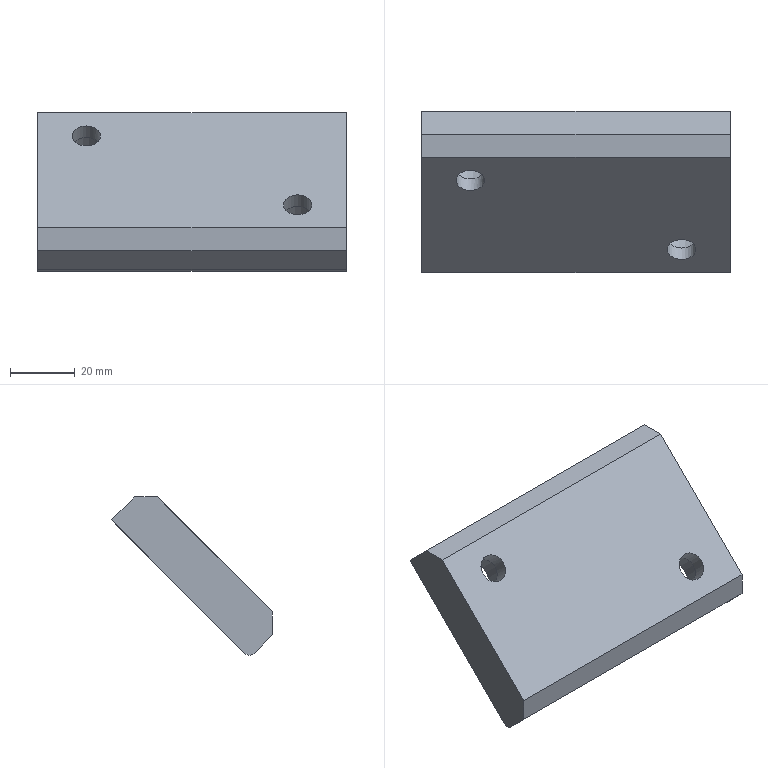Part | STEP file | 1_id1550_x_t | 1 solid | 15 faces | box 95 x 49.497 x 48.669 mm | volume 78915 mm3 | plane 10 | cylinder 5 | commonest cylinder face diameters 8.7 x2 15 x2 4 x1
STEP:
#1=CARTESIAN_POINT('',(0.,0.,0.));
#2=DIRECTION('',(0.,0.,1.));
#3=DIRECTION('',(1.,0.,0.));
#4=AXIS2_PLACEMENT_3D('',#1,#2,#3);
#5=CARTESIAN_POINT('',(700.426,19.419,-33.42));
#6=VERTEX_POINT('',#5);
#7=CARTESIAN_POINT('',(700.426,-21.593,-74.432));
#8=VERTEX_POINT('',#7);
#9=CARTESIAN_POINT('',(700.426,19.419,-33.42));
#10=DIRECTION('',(0.,-0.7071,-0.7071));
#11=VECTOR('',#10,1.);
#12=LINE('',#9,#11);
#13=CARTESIAN_POINT('',(700.426,-5.329,-26.349));
#14=DIRECTION('',(-1.,0.,0.));
#15=DIRECTION('',(0.,0.,1.));
#16=AXIS2_PLACEMENT_3D('',#13,#14,#15);
#17=PLANE('',#16);
#18=CARTESIAN_POINT('',(-7.071,24.749));
#19=DIRECTION('',(-0.7071,-0.7071));
#20=VECTOR('',#19,1.);
#21=LINE('',#18,#20);
#22=(GEOMETRIC_REPRESENTATION_CONTEXT(2)PARAMETRIC_REPRESENTATION_CONTEXT()REPRESENTATION_CONTEXT('',''));
#23=DEFINITIONAL_REPRESENTATION('',(#21),#22);
#24=PCURVE('',#17,#23);
#25=CARTESIAN_POINT('',(747.926,22.955,-29.884));
#26=DIRECTION('',(0.,-0.7071,0.7071));
#27=DIRECTION('',(0.,-0.7071,-0.7071));
#28=AXIS2_PLACEMENT_3D('',#25,#26,#27);
#29=PLANE('',#28);
#30=CARTESIAN_POINT('',(5.,-47.5));
#31=DIRECTION('',(1.,0.));
#32=VECTOR('',#31,1.);
#33=LINE('',#30,#32);
#34=(GEOMETRIC_REPRESENTATION_CONTEXT(2)PARAMETRIC_REPRESENTATION_CONTEXT()REPRESENTATION_CONTEXT('',''));
#35=DEFINITIONAL_REPRESENTATION('',(#33),#34);
#36=PCURVE('',#29,#35);
#37=SURFACE_CURVE('',#12,(#24,#36),.PCURVE_S1.);
#38=EDGE_CURVE('',#6,#8,#37,.T.);
#39=ORIENTED_EDGE('',*,*,#38,.T.);
#40=CARTESIAN_POINT('',(700.426,-24.421,-74.432));
#41=VERTEX_POINT('',#40);
#42=CARTESIAN_POINT('',(700.426,-23.007,-73.018));
#43=DIRECTION('',(-1.,0.,0.));
#44=DIRECTION('',(0.,0.,-1.));
#45=AXIS2_PLACEMENT_3D('',#42,#43,#44);
#46=CIRCLE('',#45,2.);
#47=CARTESIAN_POINT('',(-46.669,-17.678));
#48=DIRECTION('',(-1.,0.));
#49=AXIS2_PLACEMENT_2D('',#47,#48);
#50=CIRCLE('',#49,2.);
#51=(GEOMETRIC_REPRESENTATION_CONTEXT(2)PARAMETRIC_REPRESENTATION_CONTEXT()REPRESENTATION_CONTEXT('',''));
#52=DEFINITIONAL_REPRESENTATION('',(#50),#51);
#53=PCURVE('',#17,#52);
#54=CARTESIAN_POINT('',(700.426,-23.007,-73.018));
#55=DIRECTION('',(-1.,0.,0.));
#56=DIRECTION('',(0.,0.,1.));
#57=AXIS2_PLACEMENT_3D('',#54,#55,#56);
#58=CYLINDRICAL_SURFACE('',#57,2.);
#59=CARTESIAN_POINT('',(-3.142,0.));
#60=DIRECTION('',(1.,0.));
#61=VECTOR('',#60,1.);
#62=LINE('',#59,#61);
#63=(GEOMETRIC_REPRESENTATION_CONTEXT(2)PARAMETRIC_REPRESENTATION_CONTEXT()REPRESENTATION_CONTEXT('',''));
#64=DEFINITIONAL_REPRESENTATION('',(#62),#63);
#65=PCURVE('',#58,#64);
#66=SURFACE_CURVE('',#46,(#53,#65),.PCURVE_S1.);
#67=EDGE_CURVE('',#8,#41,#66,.T.);
#68=ORIENTED_EDGE('',*,*,#67,.T.);
#69=CARTESIAN_POINT('',(700.426,-30.078,-68.775));
#70=VERTEX_POINT('',#69);
#71=CARTESIAN_POINT('',(700.426,-24.421,-74.432));
#72=DIRECTION('',(0.,-0.7071,0.7071));
#73=VECTOR('',#72,1.);
#74=LINE('',#71,#73);
#75=CARTESIAN_POINT('',(-48.083,-19.092));
#76=DIRECTION('',(0.7071,-0.7071));
#77=VECTOR('',#76,1.);
#78=LINE('',#75,#77);
#79=(GEOMETRIC_REPRESENTATION_CONTEXT(2)PARAMETRIC_REPRESENTATION_CONTEXT()REPRESENTATION_CONTEXT('',''));
#80=DEFINITIONAL_REPRESENTATION('',(#78),#79);
#81=PCURVE('',#17,#80);
#82=CARTESIAN_POINT('',(700.426,-33.614,-65.239));
#83=DIRECTION('',(0.,-0.7071,-0.7071));
#84=DIRECTION('',(0.,0.7071,-0.7071));
#85=AXIS2_PLACEMENT_3D('',#82,#83,#84);
#86=PLANE('',#85);
#87=CARTESIAN_POINT('',(13.,0.));
#88=DIRECTION('',(-1.,0.));
#89=VECTOR('',#88,1.);
#90=LINE('',#87,#89);
#91=(GEOMETRIC_REPRESENTATION_CONTEXT(2)PARAMETRIC_REPRESENTATION_CONTEXT()REPRESENTATION_CONTEXT('',''));
#92=DEFINITIONAL_REPRESENTATION('',(#90),#91);
#93=PCURVE('',#86,#92);
#94=SURFACE_CURVE('',#74,(#81,#93),.PCURVE_S1.);
#95=EDGE_CURVE('',#41,#70,#94,.T.);
#96=ORIENTED_EDGE('',*,*,#95,.T.);
#97=CARTESIAN_POINT('',(700.426,-30.078,-61.704));
#98=VERTEX_POINT('',#97);
#99=CARTESIAN_POINT('',(700.426,-30.078,-68.775));
#100=DIRECTION('',(0.,0.,1.));
#101=VECTOR('',#100,1.);
#102=LINE('',#99,#101);
#103=CARTESIAN_POINT('',(-42.426,-24.749));
#104=DIRECTION('',(1.,0.));
#105=VECTOR('',#104,1.);
#106=LINE('',#103,#105);
#107=(GEOMETRIC_REPRESENTATION_CONTEXT(2)PARAMETRIC_REPRESENTATION_CONTEXT()REPRESENTATION_CONTEXT('',''));
#108=DEFINITIONAL_REPRESENTATION('',(#106),#107);
#109=PCURVE('',#17,#108);
#110=CARTESIAN_POINT('',(747.926,-30.078,-26.349));
#111=DIRECTION('',(0.,-1.,0.));
#112=DIRECTION('',(0.,0.,-1.));
#113=AXIS2_PLACEMENT_3D('',#110,#111,#112);
#114=PLANE('',#113);
#115=CARTESIAN_POINT('',(42.426,-47.5));
#116=DIRECTION('',(-1.,0.));
#117=VECTOR('',#116,1.);
#118=LINE('',#115,#117);
#119=(GEOMETRIC_REPRESENTATION_CONTEXT(2)PARAMETRIC_REPRESENTATION_CONTEXT()REPRESENTATION_CONTEXT('',''));
#120=DEFINITIONAL_REPRESENTATION('',(#118),#119);
#121=PCURVE('',#114,#120);
#122=SURFACE_CURVE('',#102,(#109,#121),.PCURVE_S1.);
#123=EDGE_CURVE('',#70,#98,#122,.T.);
#124=ORIENTED_EDGE('',*,*,#123,.T.);
#125=CARTESIAN_POINT('',(700.426,5.277,-26.349));
#126=VERTEX_POINT('',#125);
#127=CARTESIAN_POINT('',(700.426,-30.078,-61.704));
#128=DIRECTION('',(0.,0.7071,0.7071));
#129=VECTOR('',#128,1.);
#130=LINE('',#127,#129);
#131=CARTESIAN_POINT('',(-35.355,-24.749));
#132=DIRECTION('',(0.7071,0.7071));
#133=VECTOR('',#132,1.);
#134=LINE('',#131,#133);
#135=(GEOMETRIC_REPRESENTATION_CONTEXT(2)PARAMETRIC_REPRESENTATION_CONTEXT()REPRESENTATION_CONTEXT('',''));
#136=DEFINITIONAL_REPRESENTATION('',(#134),#135);
#137=PCURVE('',#17,#136);
#138=CARTESIAN_POINT('',(747.926,8.813,-22.813));
#139=DIRECTION('',(0.,-0.7071,0.7071));
#140=DIRECTION('',(0.,-0.7071,-0.7071));
#141=AXIS2_PLACEMENT_3D('',#138,#139,#140);
#142=PLANE('',#141);
#143=CARTESIAN_POINT('',(55.,-47.5));
#144=DIRECTION('',(-1.,0.));
#145=VECTOR('',#144,1.);
#146=LINE('',#143,#145);
#147=(GEOMETRIC_REPRESENTATION_CONTEXT(2)PARAMETRIC_REPRESENTATION_CONTEXT()REPRESENTATION_CONTEXT('',''));
#148=DEFINITIONAL_REPRESENTATION('',(#146),#147);
#149=PCURVE('',#142,#148);
#150=SURFACE_CURVE('',#130,(#137,#149),.PCURVE_S1.);
#151=EDGE_CURVE('',#98,#126,#150,.T.);
#152=ORIENTED_EDGE('',*,*,#151,.T.);
#153=CARTESIAN_POINT('',(700.426,12.348,-26.349));
#154=VERTEX_POINT('',#153);
#155=CARTESIAN_POINT('',(700.426,5.277,-26.349));
#156=DIRECTION('',(0.,1.,0.));
#157=VECTOR('',#156,1.);
#158=LINE('',#155,#157);
#159=CARTESIAN_POINT('',(0.,10.607));
#160=DIRECTION('',(0.,1.));
#161=VECTOR('',#160,1.);
#162=LINE('',#159,#161);
#163=(GEOMETRIC_REPRESENTATION_CONTEXT(2)PARAMETRIC_REPRESENTATION_CONTEXT()REPRESENTATION_CONTEXT('',''));
#164=DEFINITIONAL_REPRESENTATION('',(#162),#163);
#165=PCURVE('',#17,#164);
#166=CARTESIAN_POINT('',(747.926,-5.329,-26.349));
#167=DIRECTION('',(0.,0.,1.));
#168=DIRECTION('',(1.,0.,0.));
#169=AXIS2_PLACEMENT_3D('',#166,#167,#168);
#170=PLANE('',#169);
#171=CARTESIAN_POINT('',(-47.5,10.607));
#172=DIRECTION('',(0.,1.));
#173=VECTOR('',#172,1.);
#174=LINE('',#171,#173);
#175=(GEOMETRIC_REPRESENTATION_CONTEXT(2)PARAMETRIC_REPRESENTATION_CONTEXT()REPRESENTATION_CONTEXT('',''));
#176=DEFINITIONAL_REPRESENTATION('',(#174),#175);
#177=PCURVE('',#170,#176);
#178=SURFACE_CURVE('',#158,(#165,#177),.PCURVE_S1.);
#179=EDGE_CURVE('',#126,#154,#178,.T.);
#180=ORIENTED_EDGE('',*,*,#179,.T.);
#181=CARTESIAN_POINT('',(700.426,12.348,-26.349));
#182=DIRECTION('',(0.,0.7071,-0.7071));
#183=VECTOR('',#182,1.);
#184=LINE('',#181,#183);
#185=CARTESIAN_POINT('',(0.,17.678));
#186=DIRECTION('',(-0.7071,0.7071));
#187=VECTOR('',#186,1.);
#188=LINE('',#185,#187);
#189=(GEOMETRIC_REPRESENTATION_CONTEXT(2)PARAMETRIC_REPRESENTATION_CONTEXT()REPRESENTATION_CONTEXT('',''));
#190=DEFINITIONAL_REPRESENTATION('',(#188),#189);
#191=PCURVE('',#17,#190);
#192=CARTESIAN_POINT('',(795.426,8.813,-22.813));
#193=DIRECTION('',(0.,0.7071,0.7071));
#194=DIRECTION('',(-1.,0.,0.));
#195=AXIS2_PLACEMENT_3D('',#192,#193,#194);
#196=PLANE('',#195);
#197=CARTESIAN_POINT('',(95.,-5.));
#198=DIRECTION('',(0.,-1.));
#199=VECTOR('',#198,1.);
#200=LINE('',#197,#199);
#201=(GEOMETRIC_REPRESENTATION_CONTEXT(2)PARAMETRIC_REPRESENTATION_CONTEXT()REPRESENTATION_CONTEXT('',''));
#202=DEFINITIONAL_REPRESENTATION('',(#200),#201);
#203=PCURVE('',#196,#202);
#204=SURFACE_CURVE('',#184,(#191,#203),.PCURVE_S1.);
#205=EDGE_CURVE('',#154,#6,#204,.T.);
#206=ORIENTED_EDGE('',*,*,#205,.T.);
#207=EDGE_LOOP('',(#39,#68,#96,#124,#152,#180,#206));
#208=FACE_BOUND('',#207,.T.);
#209=ADVANCED_FACE('',(#208),#17,.T.);
#210=CARTESIAN_POINT('',(795.426,19.419,-33.42));
#211=VERTEX_POINT('',#210);
#212=CARTESIAN_POINT('',(700.426,19.419,-33.42));
#213=DIRECTION('',(1.,0.,0.));
#214=VECTOR('',#213,1.);
#215=LINE('',#212,#214);
#216=CARTESIAN_POINT('',(5.,-47.5));
#217=DIRECTION('',(0.,1.));
#218=VECTOR('',#217,1.);
#219=LINE('',#216,#218);
#220=(GEOMETRIC_REPRESENTATION_CONTEXT(2)PARAMETRIC_REPRESENTATION_CONTEXT()REPRESENTATION_CONTEXT('',''));
#221=DEFINITIONAL_REPRESENTATION('',(#219),#220);
#222=PCURVE('',#29,#221);
#223=CARTESIAN_POINT('',(95.,-15.));
#224=DIRECTION('',(-1.,0.));
#225=VECTOR('',#224,1.);
#226=LINE('',#223,#225);
#227=(GEOMETRIC_REPRESENTATION_CONTEXT(2)PARAMETRIC_REPRESENTATION_CONTEXT()REPRESENTATION_CONTEXT('',''));
#228=DEFINITIONAL_REPRESENTATION('',(#226),#227);
#229=PCURVE('',#196,#228);
#230=SURFACE_CURVE('',#215,(#222,#229),.PCURVE_S1.);
#231=EDGE_CURVE('',#6,#211,#230,.T.);
#232=ORIENTED_EDGE('',*,*,#231,.T.);
#233=CARTESIAN_POINT('',(795.426,-21.593,-74.432));
#234=VERTEX_POINT('',#233);
#235=CARTESIAN_POINT('',(795.426,-21.593,-74.432));
#236=DIRECTION('',(0.,0.7071,0.7071));
#237=VECTOR('',#236,1.);
#238=LINE('',#235,#237);
#239=CARTESIAN_POINT('',(63.,47.5));
#240=DIRECTION('',(-1.,0.));
#241=VECTOR('',#240,1.);
#242=LINE('',#239,#241);
#243=(GEOMETRIC_REPRESENTATION_CONTEXT(2)PARAMETRIC_REPRESENTATION_CONTEXT()REPRESENTATION_CONTEXT('',''));
#244=DEFINITIONAL_REPRESENTATION('',(#242),#243);
#245=PCURVE('',#29,#244);
#246=CARTESIAN_POINT('',(795.426,-5.329,-26.349));
#247=DIRECTION('',(1.,0.,0.));
#248=DIRECTION('',(0.,0.,-1.));
#249=AXIS2_PLACEMENT_3D('',#246,#247,#248);
#250=PLANE('',#249);
#251=CARTESIAN_POINT('',(48.083,-16.263));
#252=DIRECTION('',(-0.7071,0.7071));
#253=VECTOR('',#252,1.);
#254=LINE('',#251,#253);
#255=(GEOMETRIC_REPRESENTATION_CONTEXT(2)PARAMETRIC_REPRESENTATION_CONTEXT()REPRESENTATION_CONTEXT('',''));
#256=DEFINITIONAL_REPRESENTATION('',(#254),#255);
#257=PCURVE('',#250,#256);
#258=SURFACE_CURVE('',#238,(#245,#257),.PCURVE_S1.);
#259=EDGE_CURVE('',#234,#211,#258,.T.);
#260=ORIENTED_EDGE('',*,*,#259,.F.);
#261=CARTESIAN_POINT('',(700.426,-21.593,-74.432));
#262=DIRECTION('',(1.,0.,0.));
#263=VECTOR('',#262,1.);
#264=LINE('',#261,#263);
#265=CARTESIAN_POINT('',(63.,-47.5));
#266=DIRECTION('',(0.,1.));
#267=VECTOR('',#266,1.);
#268=LINE('',#265,#267);
#269=(GEOMETRIC_REPRESENTATION_CONTEXT(2)PARAMETRIC_REPRESENTATION_CONTEXT()REPRESENTATION_CONTEXT('',''));
#270=DEFINITIONAL_REPRESENTATION('',(#268),#269);
#271=PCURVE('',#29,#270);
#272=CARTESIAN_POINT('',(2.356,0.));
#273=DIRECTION('',(0.,-1.));
#274=VECTOR('',#273,1.);
#275=LINE('',#272,#274);
#276=(GEOMETRIC_REPRESENTATION_CONTEXT(2)PARAMETRIC_REPRESENTATION_CONTEXT()REPRESENTATION_CONTEXT('',''));
#277=DEFINITIONAL_REPRESENTATION('',(#275),#276);
#278=PCURVE('',#58,#277);
#279=SURFACE_CURVE('',#264,(#271,#278),.PCURVE_S1.);
#280=EDGE_CURVE('',#8,#234,#279,.T.);
#281=ORIENTED_EDGE('',*,*,#280,.F.);
#282=ORIENTED_EDGE('',*,*,#38,.F.);
#283=EDGE_LOOP('',(#232,#260,#281,#282));
#284=FACE_BOUND('',#283,.T.);
#285=CARTESIAN_POINT('',(772.926,-12.4,-65.239));
#286=VERTEX_POINT('',#285);
#287=CARTESIAN_POINT('',(787.926,-12.4,-65.239));
#288=VERTEX_POINT('',#287);
#289=CARTESIAN_POINT('',(780.426,-12.4,-65.239));
#290=DIRECTION('',(0.,-0.7071,0.7071));
#291=DIRECTION('',(-1.,0.,0.));
#292=AXIS2_PLACEMENT_3D('',#289,#290,#291);
#293=CIRCLE('',#292,7.5);
#294=CARTESIAN_POINT('',(50.,32.5));
#295=DIRECTION('',(0.,-1.));
#296=AXIS2_PLACEMENT_2D('',#294,#295);
#297=CIRCLE('',#296,7.5);
#298=(GEOMETRIC_REPRESENTATION_CONTEXT(2)PARAMETRIC_REPRESENTATION_CONTEXT()REPRESENTATION_CONTEXT('',''));
#299=DEFINITIONAL_REPRESENTATION('',(#297),#298);
#300=PCURVE('',#29,#299);
#301=CARTESIAN_POINT('',(780.426,-19.471,-58.168));
#302=DIRECTION('',(0.,-0.7071,0.7071));
#303=DIRECTION('',(1.,0.,0.));
#304=AXIS2_PLACEMENT_3D('',#301,#302,#303);
#305=CYLINDRICAL_SURFACE('',#304,7.5);
#306=CARTESIAN_POINT('',(3.142,-10.));
#307=DIRECTION('',(1.,0.));
#308=VECTOR('',#307,1.);
#309=LINE('',#306,#308);
#310=(GEOMETRIC_REPRESENTATION_CONTEXT(2)PARAMETRIC_REPRESENTATION_CONTEXT()REPRESENTATION_CONTEXT('',''));
#311=DEFINITIONAL_REPRESENTATION('',(#309),#310);
#312=PCURVE('',#305,#311);
#313=SURFACE_CURVE('',#293,(#300,#312),.PCURVE_S1.);
#314=EDGE_CURVE('',#286,#288,#313,.T.);
#315=ORIENTED_EDGE('',*,*,#314,.T.);
#316=CARTESIAN_POINT('',(780.426,-12.4,-65.239));
#317=DIRECTION('',(0.,-0.7071,0.7071));
#318=DIRECTION('',(-1.,0.,0.));
#319=AXIS2_PLACEMENT_3D('',#316,#317,#318);
#320=CIRCLE('',#319,7.5);
#321=CARTESIAN_POINT('',(50.,32.5));
#322=DIRECTION('',(0.,-1.));
#323=AXIS2_PLACEMENT_2D('',#321,#322);
#324=CIRCLE('',#323,7.5);
#325=(GEOMETRIC_REPRESENTATION_CONTEXT(2)PARAMETRIC_REPRESENTATION_CONTEXT()REPRESENTATION_CONTEXT('',''));
#326=DEFINITIONAL_REPRESENTATION('',(#324),#325);
#327=PCURVE('',#29,#326);
#328=CARTESIAN_POINT('',(-3.142,-10.));
#329=DIRECTION('',(1.,0.));
#330=VECTOR('',#329,1.);
#331=LINE('',#328,#330);
#332=(GEOMETRIC_REPRESENTATION_CONTEXT(2)PARAMETRIC_REPRESENTATION_CONTEXT()REPRESENTATION_CONTEXT('',''));
#333=DEFINITIONAL_REPRESENTATION('',(#331),#332);
#334=PCURVE('',#305,#333);
#335=SURFACE_CURVE('',#320,(#327,#334),.PCURVE_S1.);
#336=EDGE_CURVE('',#288,#286,#335,.T.);
#337=ORIENTED_EDGE('',*,*,#336,.T.);
#338=EDGE_LOOP('',(#315,#337));
#339=FACE_BOUND('',#338,.T.);
#340=CARTESIAN_POINT('',(722.926,8.813,-44.026));
#341=VERTEX_POINT('',#340);
#342=CARTESIAN_POINT('',(715.426,8.813,-44.026));
#343=DIRECTION('',(0.,-0.7071,0.7071));
#344=DIRECTION('',(1.,0.,0.));
#345=AXIS2_PLACEMENT_3D('',#342,#343,#344);
#346=CIRCLE('',#345,7.5);
#347=CARTESIAN_POINT('',(20.,-32.5));
#348=DIRECTION('',(0.,1.));
#349=AXIS2_PLACEMENT_2D('',#347,#348);
#350=CIRCLE('',#349,7.5);
#351=(GEOMETRIC_REPRESENTATION_CONTEXT(2)PARAMETRIC_REPRESENTATION_CONTEXT()REPRESENTATION_CONTEXT('',''));
#352=DEFINITIONAL_REPRESENTATION('',(#350),#351);
#353=PCURVE('',#29,#352);
#354=CARTESIAN_POINT('',(715.426,1.742,-36.955));
#355=DIRECTION('',(0.,-0.7071,0.7071));
#356=DIRECTION('',(-1.,0.,0.));
#357=AXIS2_PLACEMENT_3D('',#354,#355,#356);
#358=CYLINDRICAL_SURFACE('',#357,7.5);
#359=CARTESIAN_POINT('',(3.142,-10.));
#360=DIRECTION('',(1.,0.));
#361=VECTOR('',#360,1.);
#362=LINE('',#359,#361);
#363=(GEOMETRIC_REPRESENTATION_CONTEXT(2)PARAMETRIC_REPRESENTATION_CONTEXT()REPRESENTATION_CONTEXT('',''));
#364=DEFINITIONAL_REPRESENTATION('',(#362),#363);
#365=PCURVE('',#358,#364);
#366=SURFACE_CURVE('',#346,(#353,#365),.PCURVE_S1.);
#367=EDGE_CURVE('',#341,#341,#366,.T.);
#368=ORIENTED_EDGE('',*,*,#367,.T.);
#369=EDGE_LOOP('',(#368));
#370=FACE_BOUND('',#369,.T.);
#371=ADVANCED_FACE('',(#284,#339,#370),#29,.F.);
#372=CARTESIAN_POINT('',(787.926,-19.471,-58.168));
#373=VERTEX_POINT('',#372);
#374=CARTESIAN_POINT('',(780.426,-19.471,-58.168));
#375=DIRECTION('',(0.,0.7071,-0.7071));
#376=DIRECTION('',(1.,0.,0.));
#377=AXIS2_PLACEMENT_3D('',#374,#375,#376);
#378=CIRCLE('',#377,7.5);
#379=CARTESIAN_POINT('',(6.283,0.));
#380=DIRECTION('',(-1.,0.));
#381=VECTOR('',#380,1.);
#382=LINE('',#379,#381);
#383=(GEOMETRIC_REPRESENTATION_CONTEXT(2)PARAMETRIC_REPRESENTATION_CONTEXT()REPRESENTATION_CONTEXT('',''));
#384=DEFINITIONAL_REPRESENTATION('',(#382),#383);
#385=PCURVE('',#305,#384);
#386=CARTESIAN_POINT('',(780.426,-19.471,-58.168));
#387=DIRECTION('',(0.,-0.7071,0.7071));
#388=DIRECTION('',(1.,0.,0.));
#389=AXIS2_PLACEMENT_3D('',#386,#387,#388);
#390=PLANE('',#389);
#391=CARTESIAN_POINT('',(7.5,0.));
#392=CARTESIAN_POINT('',(7.5,-12.99));
#393=CARTESIAN_POINT('',(-3.75,-6.495));
#394=CARTESIAN_POINT('',(-15.,0.));
#395=CARTESIAN_POINT('',(-3.75,6.495));
#396=CARTESIAN_POINT('',(7.5,12.99));
#397=CARTESIAN_POINT('',(7.5,0.));
#398=(BOUNDED_CURVE()B_SPLINE_CURVE(2,(#391,#392,#393,#394,#395,#396,#397),.UNSPECIFIED.,.T.,.F.)B_SPLINE_CURVE_WITH_KNOTS((1,2,2,2,2,1),(-2.094,0.,2.094,4.189,6.283,8.378),.UNSPECIFIED.)CURVE()GEOMETRIC_REPRESENTATION_ITEM()RATIONAL_B_SPLINE_CURVE((1.,0.5,1.,0.5,1.,0.5,1.))REPRESENTATION_ITEM(''));
#399=(GEOMETRIC_REPRESENTATION_CONTEXT(2)PARAMETRIC_REPRESENTATION_CONTEXT()REPRESENTATION_CONTEXT('',''));
#400=DEFINITIONAL_REPRESENTATION('',(#398),#399);
#401=PCURVE('',#390,#400);
#402=SURFACE_CURVE('',#378,(#385,#401),.PCURVE_S1.);
#403=EDGE_CURVE('',#373,#373,#402,.T.);
#404=ORIENTED_EDGE('',*,*,#403,.T.);
#405=CARTESIAN_POINT('',(787.926,-12.4,-65.239));
#406=CARTESIAN_POINT('',(787.926,-19.471,-58.168));
#407=B_SPLINE_CURVE_WITH_KNOTS('',1,(#405,#406),.UNSPECIFIED.,.F.,.F.,(2,2),(-10.,0.),.PIECEWISE_BEZIER_KNOTS.);
#408=CARTESIAN_POINT('',(0.,0.));
#409=DIRECTION('',(0.,1.));
#410=VECTOR('',#409,1.);
#411=LINE('',#408,#410);
#412=(GEOMETRIC_REPRESENTATION_CONTEXT(2)PARAMETRIC_REPRESENTATION_CONTEXT()REPRESENTATION_CONTEXT('',''));
#413=DEFINITIONAL_REPRESENTATION('',(#411),#412);
#414=PCURVE('',#305,#413);
#415=CARTESIAN_POINT('',(6.283,0.));
#416=DIRECTION('',(0.,1.));
#417=VECTOR('',#416,1.);
#418=LINE('',#415,#417);
#419=(GEOMETRIC_REPRESENTATION_CONTEXT(2)PARAMETRIC_REPRESENTATION_CONTEXT()REPRESENTATION_CONTEXT('',''));
#420=DEFINITIONAL_REPRESENTATION('',(#418),#419);
#421=PCURVE('',#305,#420);
#422=SEAM_CURVE('',#407,(#414,#421),.PCURVE_S1.);
#423=EDGE_CURVE('',#288,#373,#422,.T.);
#424=ORIENTED_EDGE('',*,*,#423,.F.);
#425=ORIENTED_EDGE('',*,*,#336,.T.);
#426=ORIENTED_EDGE('',*,*,#314,.T.);
#427=ORIENTED_EDGE('',*,*,#423,.T.);
#428=EDGE_LOOP('',(#404,#424,#425,#426,#427));
#429=FACE_BOUND('',#428,.F.);
#430=ADVANCED_FACE('',(#429),#305,.F.);
#431=ORIENTED_EDGE('',*,*,#403,.T.);
#432=EDGE_LOOP('',(#431));
#433=FACE_BOUND('',#432,.T.);
#434=CARTESIAN_POINT('',(780.426,-22.547,-61.244));
#435=VERTEX_POINT('',#434);
#436=CARTESIAN_POINT('',(780.426,-19.471,-58.168));
#437=DIRECTION('',(0.,-0.7071,0.7071));
#438=DIRECTION('',(0.,-0.7071,-0.7071));
#439=AXIS2_PLACEMENT_3D('',#436,#437,#438);
#440=CIRCLE('',#439,4.35);
#441=CARTESIAN_POINT('',(0.,0.));
#442=DIRECTION('',(0.,-1.));
#443=AXIS2_PLACEMENT_2D('',#441,#442);
#444=CIRCLE('',#443,4.35);
#445=(GEOMETRIC_REPRESENTATION_CONTEXT(2)PARAMETRIC_REPRESENTATION_CONTEXT()REPRESENTATION_CONTEXT('',''));
#446=DEFINITIONAL_REPRESENTATION('',(#444),#445);
#447=PCURVE('',#390,#446);
#448=CARTESIAN_POINT('',(780.426,-23.113,-54.527));
#449=DIRECTION('',(0.,-0.7071,0.7071));
#450=DIRECTION('',(1.,0.,0.));
#451=AXIS2_PLACEMENT_3D('',#448,#449,#450);
#452=CYLINDRICAL_SURFACE('',#451,4.35);
#453=CARTESIAN_POINT('',(4.712,-5.15));
#454=DIRECTION('',(1.,0.));
#455=VECTOR('',#454,1.);
#456=LINE('',#453,#455);
#457=(GEOMETRIC_REPRESENTATION_CONTEXT(2)PARAMETRIC_REPRESENTATION_CONTEXT()REPRESENTATION_CONTEXT('',''));
#458=DEFINITIONAL_REPRESENTATION('',(#456),#457);
#459=PCURVE('',#452,#458);
#460=SURFACE_CURVE('',#440,(#447,#459),.PCURVE_S1.);
#461=EDGE_CURVE('',#435,#435,#460,.T.);
#462=ORIENTED_EDGE('',*,*,#461,.T.);
#463=EDGE_LOOP('',(#462));
#464=FACE_BOUND('',#463,.T.);
#465=ADVANCED_FACE('',(#433,#464),#390,.F.);
#466=CARTESIAN_POINT('',(780.426,-26.083,-57.709));
#467=VERTEX_POINT('',#466);
#468=CARTESIAN_POINT('',(780.426,-23.007,-54.633));
#469=DIRECTION('',(0.,0.7071,-0.7071));
#470=DIRECTION('',(0.,-0.7071,-0.7071));
#471=AXIS2_PLACEMENT_3D('',#468,#469,#470);
#472=CIRCLE('',#471,4.35);
#473=CARTESIAN_POINT('',(10.996,-0.15));
#474=DIRECTION('',(-1.,0.));
#475=VECTOR('',#474,1.);
#476=LINE('',#473,#475);
#477=(GEOMETRIC_REPRESENTATION_CONTEXT(2)PARAMETRIC_REPRESENTATION_CONTEXT()REPRESENTATION_CONTEXT('',''));
#478=DEFINITIONAL_REPRESENTATION('',(#476),#477);
#479=PCURVE('',#452,#478);
#480=CARTESIAN_POINT('',(49.35,32.5));
#481=CARTESIAN_POINT('',(49.35,24.966));
#482=CARTESIAN_POINT('',(42.825,28.733));
#483=CARTESIAN_POINT('',(36.3,32.5));
#484=CARTESIAN_POINT('',(42.825,36.267));
#485=CARTESIAN_POINT('',(49.35,40.034));
#486=CARTESIAN_POINT('',(49.35,32.5));
#487=(BOUNDED_CURVE()B_SPLINE_CURVE(2,(#480,#481,#482,#483,#484,#485,#486),.UNSPECIFIED.,.T.,.F.)B_SPLINE_CURVE_WITH_KNOTS((1,2,2,2,2,1),(-2.094,0.,2.094,4.189,6.283,8.378),.UNSPECIFIED.)CURVE()GEOMETRIC_REPRESENTATION_ITEM()RATIONAL_B_SPLINE_CURVE((1.,0.5,1.,0.5,1.,0.5,1.))REPRESENTATION_ITEM(''));
#488=(GEOMETRIC_REPRESENTATION_CONTEXT(2)PARAMETRIC_REPRESENTATION_CONTEXT()REPRESENTATION_CONTEXT('',''));
#489=DEFINITIONAL_REPRESENTATION('',(#487),#488);
#490=PCURVE('',#142,#489);
#491=SURFACE_CURVE('',#472,(#479,#490),.PCURVE_S1.);
#492=EDGE_CURVE('',#467,#467,#491,.T.);
#493=ORIENTED_EDGE('',*,*,#492,.T.);
#494=CARTESIAN_POINT('',(780.426,-22.547,-61.244));
#495=CARTESIAN_POINT('',(780.426,-26.083,-57.709));
#496=B_SPLINE_CURVE_WITH_KNOTS('',1,(#494,#495),.UNSPECIFIED.,.F.,.F.,(2,2),(-5.15,-0.15),.PIECEWISE_BEZIER_KNOTS.);
#497=CARTESIAN_POINT('',(4.712,0.));
#498=DIRECTION('',(0.,1.));
#499=VECTOR('',#498,1.);
#500=LINE('',#497,#499);
#501=(GEOMETRIC_REPRESENTATION_CONTEXT(2)PARAMETRIC_REPRESENTATION_CONTEXT()REPRESENTATION_CONTEXT('',''));
#502=DEFINITIONAL_REPRESENTATION('',(#500),#501);
#503=PCURVE('',#452,#502);
#504=CARTESIAN_POINT('',(10.996,0.));
#505=DIRECTION('',(0.,1.));
#506=VECTOR('',#505,1.);
#507=LINE('',#504,#506);
#508=(GEOMETRIC_REPRESENTATION_CONTEXT(2)PARAMETRIC_REPRESENTATION_CONTEXT()REPRESENTATION_CONTEXT('',''));
#509=DEFINITIONAL_REPRESENTATION('',(#507),#508);
#510=PCURVE('',#452,#509);
#511=SEAM_CURVE('',#496,(#503,#510),.PCURVE_S1.);
#512=EDGE_CURVE('',#435,#467,#511,.T.);
#513=ORIENTED_EDGE('',*,*,#512,.F.);
#514=ORIENTED_EDGE('',*,*,#461,.T.);
#515=ORIENTED_EDGE('',*,*,#512,.T.);
#516=EDGE_LOOP('',(#493,#513,#514,#515));
#517=FACE_BOUND('',#516,.F.);
#518=ADVANCED_FACE('',(#517),#452,.F.);
#519=CARTESIAN_POINT('',(795.426,5.277,-26.349));
#520=VERTEX_POINT('',#519);
#521=CARTESIAN_POINT('',(795.426,-30.078,-61.704));
#522=VERTEX_POINT('',#521);
#523=CARTESIAN_POINT('',(795.426,5.277,-26.349));
#524=DIRECTION('',(0.,-0.7071,-0.7071));
#525=VECTOR('',#524,1.);
#526=LINE('',#523,#525);
#527=CARTESIAN_POINT('',(5.,47.5));
#528=DIRECTION('',(1.,0.));
#529=VECTOR('',#528,1.);
#530=LINE('',#527,#529);
#531=(GEOMETRIC_REPRESENTATION_CONTEXT(2)PARAMETRIC_REPRESENTATION_CONTEXT()REPRESENTATION_CONTEXT('',''));
#532=DEFINITIONAL_REPRESENTATION('',(#530),#531);
#533=PCURVE('',#142,#532);
#534=CARTESIAN_POINT('',(0.,10.607));
#535=DIRECTION('',(0.7071,-0.7071));
#536=VECTOR('',#535,1.);
#537=LINE('',#534,#536);
#538=(GEOMETRIC_REPRESENTATION_CONTEXT(2)PARAMETRIC_REPRESENTATION_CONTEXT()REPRESENTATION_CONTEXT('',''));
#539=DEFINITIONAL_REPRESENTATION('',(#537),#538);
#540=PCURVE('',#250,#539);
#541=SURFACE_CURVE('',#526,(#533,#540),.PCURVE_S1.);
#542=EDGE_CURVE('',#520,#522,#541,.T.);
#543=ORIENTED_EDGE('',*,*,#542,.F.);
#544=CARTESIAN_POINT('',(700.426,5.277,-26.349));
#545=DIRECTION('',(1.,0.,0.));
#546=VECTOR('',#545,1.);
#547=LINE('',#544,#546);
#548=CARTESIAN_POINT('',(5.,-47.5));
#549=DIRECTION('',(0.,1.));
#550=VECTOR('',#549,1.);
#551=LINE('',#548,#550);
#552=(GEOMETRIC_REPRESENTATION_CONTEXT(2)PARAMETRIC_REPRESENTATION_CONTEXT()REPRESENTATION_CONTEXT('',''));
#553=DEFINITIONAL_REPRESENTATION('',(#551),#552);
#554=PCURVE('',#142,#553);
#555=CARTESIAN_POINT('',(-47.5,10.607));
#556=DIRECTION('',(1.,0.));
#557=VECTOR('',#556,1.);
#558=LINE('',#555,#557);
#559=(GEOMETRIC_REPRESENTATION_CONTEXT(2)PARAMETRIC_REPRESENTATION_CONTEXT()REPRESENTATION_CONTEXT('',''));
#560=DEFINITIONAL_REPRESENTATION('',(#558),#559);
#561=PCURVE('',#170,#560);
#562=SURFACE_CURVE('',#547,(#554,#561),.PCURVE_S1.);
#563=EDGE_CURVE('',#126,#520,#562,.T.);
#564=ORIENTED_EDGE('',*,*,#563,.F.);
#565=ORIENTED_EDGE('',*,*,#151,.F.);
#566=CARTESIAN_POINT('',(795.426,-30.078,-61.704));
#567=DIRECTION('',(-1.,0.,0.));
#568=VECTOR('',#567,1.);
#569=LINE('',#566,#568);
#570=CARTESIAN_POINT('',(55.,47.5));
#571=DIRECTION('',(0.,-1.));
#572=VECTOR('',#571,1.);
#573=LINE('',#570,#572);
#574=(GEOMETRIC_REPRESENTATION_CONTEXT(2)PARAMETRIC_REPRESENTATION_CONTEXT()REPRESENTATION_CONTEXT('',''));
#575=DEFINITIONAL_REPRESENTATION('',(#573),#574);
#576=PCURVE('',#142,#575);
#577=CARTESIAN_POINT('',(35.355,47.5));
#578=DIRECTION('',(0.,-1.));
#579=VECTOR('',#578,1.);
#580=LINE('',#577,#579);
#581=(GEOMETRIC_REPRESENTATION_CONTEXT(2)PARAMETRIC_REPRESENTATION_CONTEXT()REPRESENTATION_CONTEXT('',''));
#582=DEFINITIONAL_REPRESENTATION('',(#580),#581);
#583=PCURVE('',#114,#582);
#584=SURFACE_CURVE('',#569,(#576,#583),.PCURVE_S1.);
#585=EDGE_CURVE('',#522,#98,#584,.T.);
#586=ORIENTED_EDGE('',*,*,#585,.F.);
#587=EDGE_LOOP('',(#543,#564,#565,#586));
#588=FACE_BOUND('',#587,.T.);
#589=ORIENTED_EDGE('',*,*,#492,.T.);
#590=EDGE_LOOP('',(#589));
#591=FACE_BOUND('',#590,.T.);
#592=CARTESIAN_POINT('',(715.426,1.282,-30.344));
#593=VERTEX_POINT('',#592);
#594=CARTESIAN_POINT('',(715.426,-1.794,-33.42));
#595=DIRECTION('',(0.,0.7071,-0.7071));
#596=DIRECTION('',(0.,0.7071,0.7071));
#597=AXIS2_PLACEMENT_3D('',#594,#595,#596);
#598=CIRCLE('',#597,4.35);
#599=CARTESIAN_POINT('',(10.65,-32.5));
#600=CARTESIAN_POINT('',(10.65,-24.966));
#601=CARTESIAN_POINT('',(17.175,-28.733));
#602=CARTESIAN_POINT('',(23.7,-32.5));
#603=CARTESIAN_POINT('',(17.175,-36.267));
#604=CARTESIAN_POINT('',(10.65,-40.034));
#605=CARTESIAN_POINT('',(10.65,-32.5));
#606=(BOUNDED_CURVE()B_SPLINE_CURVE(2,(#599,#600,#601,#602,#603,#604,#605),.UNSPECIFIED.,.T.,.F.)B_SPLINE_CURVE_WITH_KNOTS((1,2,2,2,2,1),(-2.094,0.,2.094,4.189,6.283,8.378),.UNSPECIFIED.)CURVE()GEOMETRIC_REPRESENTATION_ITEM()RATIONAL_B_SPLINE_CURVE((1.,0.5,1.,0.5,1.,0.5,1.))REPRESENTATION_ITEM(''));
#607=(GEOMETRIC_REPRESENTATION_CONTEXT(2)PARAMETRIC_REPRESENTATION_CONTEXT()REPRESENTATION_CONTEXT('',''));
#608=DEFINITIONAL_REPRESENTATION('',(#606),#607);
#609=PCURVE('',#142,#608);
#610=CARTESIAN_POINT('',(715.426,-1.9,-33.314));
#611=DIRECTION('',(0.,-0.7071,0.7071));
#612=DIRECTION('',(-1.,0.,0.));
#613=AXIS2_PLACEMENT_3D('',#610,#611,#612);
#614=CYLINDRICAL_SURFACE('',#613,4.35);
#615=CARTESIAN_POINT('',(10.996,-0.15));
#616=DIRECTION('',(-1.,0.));
#617=VECTOR('',#616,1.);
#618=LINE('',#615,#617);
#619=(GEOMETRIC_REPRESENTATION_CONTEXT(2)PARAMETRIC_REPRESENTATION_CONTEXT()REPRESENTATION_CONTEXT('',''));
#620=DEFINITIONAL_REPRESENTATION('',(#618),#619);
#621=PCURVE('',#614,#620);
#622=SURFACE_CURVE('',#598,(#609,#621),.PCURVE_S1.);
#623=EDGE_CURVE('',#593,#593,#622,.T.);
#624=ORIENTED_EDGE('',*,*,#623,.T.);
#625=EDGE_LOOP('',(#624));
#626=FACE_BOUND('',#625,.T.);
#627=ADVANCED_FACE('',(#588,#591,#626),#142,.T.);
#628=ORIENTED_EDGE('',*,*,#623,.T.);
#629=CARTESIAN_POINT('',(715.426,4.818,-33.879));
#630=VERTEX_POINT('',#629);
#631=CARTESIAN_POINT('',(715.426,4.818,-33.879));
#632=CARTESIAN_POINT('',(715.426,1.282,-30.344));
#633=B_SPLINE_CURVE_WITH_KNOTS('',1,(#631,#632),.UNSPECIFIED.,.F.,.F.,(2,2),(-5.15,-0.15),.PIECEWISE_BEZIER_KNOTS.);
#634=CARTESIAN_POINT('',(4.712,0.));
#635=DIRECTION('',(0.,1.));
#636=VECTOR('',#635,1.);
#637=LINE('',#634,#636);
#638=(GEOMETRIC_REPRESENTATION_CONTEXT(2)PARAMETRIC_REPRESENTATION_CONTEXT()REPRESENTATION_CONTEXT('',''));
#639=DEFINITIONAL_REPRESENTATION('',(#637),#638);
#640=PCURVE('',#614,#639);
#641=CARTESIAN_POINT('',(10.996,0.));
#642=DIRECTION('',(0.,1.));
#643=VECTOR('',#642,1.);
#644=LINE('',#641,#643);
#645=(GEOMETRIC_REPRESENTATION_CONTEXT(2)PARAMETRIC_REPRESENTATION_CONTEXT()REPRESENTATION_CONTEXT('',''));
#646=DEFINITIONAL_REPRESENTATION('',(#644),#645);
#647=PCURVE('',#614,#646);
#648=SEAM_CURVE('',#633,(#640,#647),.PCURVE_S1.);
#649=EDGE_CURVE('',#630,#593,#648,.T.);
#650=ORIENTED_EDGE('',*,*,#649,.F.);
#651=CARTESIAN_POINT('',(719.776,1.742,-36.955));
#652=VERTEX_POINT('',#651);
#653=CARTESIAN_POINT('',(715.426,1.742,-36.955));
#654=DIRECTION('',(0.,-0.7071,0.7071));
#655=DIRECTION('',(1.,0.,0.));
#656=AXIS2_PLACEMENT_3D('',#653,#654,#655);
#657=CIRCLE('',#656,4.35);
#658=CARTESIAN_POINT('',(3.142,-5.15));
#659=DIRECTION('',(1.,0.));
#660=VECTOR('',#659,1.);
#661=LINE('',#658,#660);
#662=(GEOMETRIC_REPRESENTATION_CONTEXT(2)PARAMETRIC_REPRESENTATION_CONTEXT()REPRESENTATION_CONTEXT('',''));
#663=DEFINITIONAL_REPRESENTATION('',(#661),#662);
#664=PCURVE('',#614,#663);
#665=CARTESIAN_POINT('',(715.426,1.742,-36.955));
#666=DIRECTION('',(0.,-0.7071,0.7071));
#667=DIRECTION('',(1.,0.,0.));
#668=AXIS2_PLACEMENT_3D('',#665,#666,#667);
#669=PLANE('',#668);
#670=CARTESIAN_POINT('',(0.,0.));
#671=DIRECTION('',(1.,0.));
#672=AXIS2_PLACEMENT_2D('',#670,#671);
#673=CIRCLE('',#672,4.35);
#674=(GEOMETRIC_REPRESENTATION_CONTEXT(2)PARAMETRIC_REPRESENTATION_CONTEXT()REPRESENTATION_CONTEXT('',''));
#675=DEFINITIONAL_REPRESENTATION('',(#673),#674);
#676=PCURVE('',#669,#675);
#677=SURFACE_CURVE('',#657,(#664,#676),.PCURVE_S1.);
#678=EDGE_CURVE('',#630,#652,#677,.T.);
#679=ORIENTED_EDGE('',*,*,#678,.T.);
#680=CARTESIAN_POINT('',(715.426,1.742,-36.955));
#681=DIRECTION('',(0.,-0.7071,0.7071));
#682=DIRECTION('',(1.,0.,0.));
#683=AXIS2_PLACEMENT_3D('',#680,#681,#682);
#684=CIRCLE('',#683,4.35);
#685=CARTESIAN_POINT('',(9.425,-5.15));
#686=DIRECTION('',(1.,0.));
#687=VECTOR('',#686,1.);
#688=LINE('',#685,#687);
#689=(GEOMETRIC_REPRESENTATION_CONTEXT(2)PARAMETRIC_REPRESENTATION_CONTEXT()REPRESENTATION_CONTEXT('',''));
#690=DEFINITIONAL_REPRESENTATION('',(#688),#689);
#691=PCURVE('',#614,#690);
#692=CARTESIAN_POINT('',(0.,0.));
#693=DIRECTION('',(1.,0.));
#694=AXIS2_PLACEMENT_2D('',#692,#693);
#695=CIRCLE('',#694,4.35);
#696=(GEOMETRIC_REPRESENTATION_CONTEXT(2)PARAMETRIC_REPRESENTATION_CONTEXT()REPRESENTATION_CONTEXT('',''));
#697=DEFINITIONAL_REPRESENTATION('',(#695),#696);
#698=PCURVE('',#669,#697);
#699=SURFACE_CURVE('',#684,(#691,#698),.PCURVE_S1.);
#700=EDGE_CURVE('',#652,#630,#699,.T.);
#701=ORIENTED_EDGE('',*,*,#700,.T.);
#702=ORIENTED_EDGE('',*,*,#649,.T.);
#703=EDGE_LOOP('',(#628,#650,#679,#701,#702));
#704=FACE_BOUND('',#703,.F.);
#705=ADVANCED_FACE('',(#704),#614,.F.);
#706=CARTESIAN_POINT('',(722.926,1.742,-36.955));
#707=VERTEX_POINT('',#706);
#708=CARTESIAN_POINT('',(715.426,1.742,-36.955));
#709=DIRECTION('',(0.,0.7071,-0.7071));
#710=DIRECTION('',(1.,0.,0.));
#711=AXIS2_PLACEMENT_3D('',#708,#709,#710);
#712=CIRCLE('',#711,7.5);
#713=CARTESIAN_POINT('',(7.5,0.));
#714=CARTESIAN_POINT('',(7.5,-12.99));
#715=CARTESIAN_POINT('',(-3.75,-6.495));
#716=CARTESIAN_POINT('',(-15.,0.));
#717=CARTESIAN_POINT('',(-3.75,6.495));
#718=CARTESIAN_POINT('',(7.5,12.99));
#719=CARTESIAN_POINT('',(7.5,0.));
#720=(BOUNDED_CURVE()B_SPLINE_CURVE(2,(#713,#714,#715,#716,#717,#718,#719),.UNSPECIFIED.,.T.,.F.)B_SPLINE_CURVE_WITH_KNOTS((1,2,2,2,2,1),(-2.094,0.,2.094,4.189,6.283,8.378),.UNSPECIFIED.)CURVE()GEOMETRIC_REPRESENTATION_ITEM()RATIONAL_B_SPLINE_CURVE((1.,0.5,1.,0.5,1.,0.5,1.))REPRESENTATION_ITEM(''));
#721=(GEOMETRIC_REPRESENTATION_CONTEXT(2)PARAMETRIC_REPRESENTATION_CONTEXT()REPRESENTATION_CONTEXT('',''));
#722=DEFINITIONAL_REPRESENTATION('',(#720),#721);
#723=PCURVE('',#669,#722);
#724=CARTESIAN_POINT('',(9.425,0.));
#725=DIRECTION('',(-1.,0.));
#726=VECTOR('',#725,1.);
#727=LINE('',#724,#726);
#728=(GEOMETRIC_REPRESENTATION_CONTEXT(2)PARAMETRIC_REPRESENTATION_CONTEXT()REPRESENTATION_CONTEXT('',''));
#729=DEFINITIONAL_REPRESENTATION('',(#727),#728);
#730=PCURVE('',#358,#729);
#731=SURFACE_CURVE('',#712,(#723,#730),.PCURVE_S1.);
#732=EDGE_CURVE('',#707,#707,#731,.T.);
#733=ORIENTED_EDGE('',*,*,#732,.T.);
#734=EDGE_LOOP('',(#733));
#735=FACE_BOUND('',#734,.T.);
#736=ORIENTED_EDGE('',*,*,#700,.T.);
#737=ORIENTED_EDGE('',*,*,#678,.T.);
#738=EDGE_LOOP('',(#736,#737));
#739=FACE_BOUND('',#738,.T.);
#740=ADVANCED_FACE('',(#735,#739),#669,.F.);
#741=ORIENTED_EDGE('',*,*,#732,.T.);
#742=CARTESIAN_POINT('',(722.926,8.813,-44.026));
#743=CARTESIAN_POINT('',(722.926,1.742,-36.955));
#744=B_SPLINE_CURVE_WITH_KNOTS('',1,(#742,#743),.UNSPECIFIED.,.F.,.F.,(2,2),(-10.,0.),.PIECEWISE_BEZIER_KNOTS.);
#745=CARTESIAN_POINT('',(3.142,0.));
#746=DIRECTION('',(0.,1.));
#747=VECTOR('',#746,1.);
#748=LINE('',#745,#747);
#749=(GEOMETRIC_REPRESENTATION_CONTEXT(2)PARAMETRIC_REPRESENTATION_CONTEXT()REPRESENTATION_CONTEXT('',''));
#750=DEFINITIONAL_REPRESENTATION('',(#748),#749);
#751=PCURVE('',#358,#750);
#752=CARTESIAN_POINT('',(9.425,0.));
#753=DIRECTION('',(0.,1.));
#754=VECTOR('',#753,1.);
#755=LINE('',#752,#754);
#756=(GEOMETRIC_REPRESENTATION_CONTEXT(2)PARAMETRIC_REPRESENTATION_CONTEXT()REPRESENTATION_CONTEXT('',''));
#757=DEFINITIONAL_REPRESENTATION('',(#755),#756);
#758=PCURVE('',#358,#757);
#759=SEAM_CURVE('',#744,(#751,#758),.PCURVE_S1.);
#760=EDGE_CURVE('',#341,#707,#759,.T.);
#761=ORIENTED_EDGE('',*,*,#760,.F.);
#762=ORIENTED_EDGE('',*,*,#367,.T.);
#763=ORIENTED_EDGE('',*,*,#760,.T.);
#764=EDGE_LOOP('',(#741,#761,#762,#763));
#765=FACE_BOUND('',#764,.F.);
#766=ADVANCED_FACE('',(#765),#358,.F.);
#767=CARTESIAN_POINT('',(795.426,-30.078,-68.775));
#768=VERTEX_POINT('',#767);
#769=CARTESIAN_POINT('',(795.426,-30.078,-68.775));
#770=DIRECTION('',(0.,0.,1.));
#771=VECTOR('',#770,1.);
#772=LINE('',#769,#771);
#773=CARTESIAN_POINT('',(42.426,47.5));
#774=DIRECTION('',(-1.,0.));
#775=VECTOR('',#774,1.);
#776=LINE('',#773,#775);
#777=(GEOMETRIC_REPRESENTATION_CONTEXT(2)PARAMETRIC_REPRESENTATION_CONTEXT()REPRESENTATION_CONTEXT('',''));
#778=DEFINITIONAL_REPRESENTATION('',(#776),#777);
#779=PCURVE('',#114,#778);
#780=CARTESIAN_POINT('',(42.426,-24.749));
#781=DIRECTION('',(-1.,0.));
#782=VECTOR('',#781,1.);
#783=LINE('',#780,#782);
#784=(GEOMETRIC_REPRESENTATION_CONTEXT(2)PARAMETRIC_REPRESENTATION_CONTEXT()REPRESENTATION_CONTEXT('',''));
#785=DEFINITIONAL_REPRESENTATION('',(#783),#784);
#786=PCURVE('',#250,#785);
#787=SURFACE_CURVE('',#772,(#779,#786),.PCURVE_S1.);
#788=EDGE_CURVE('',#768,#522,#787,.T.);
#789=ORIENTED_EDGE('',*,*,#788,.T.);
#790=ORIENTED_EDGE('',*,*,#585,.T.);
#791=ORIENTED_EDGE('',*,*,#123,.F.);
#792=CARTESIAN_POINT('',(795.426,-30.078,-68.775));
#793=DIRECTION('',(-1.,0.,0.));
#794=VECTOR('',#793,1.);
#795=LINE('',#792,#794);
#796=CARTESIAN_POINT('',(42.426,47.5));
#797=DIRECTION('',(0.,-1.));
#798=VECTOR('',#797,1.);
#799=LINE('',#796,#798);
#800=(GEOMETRIC_REPRESENTATION_CONTEXT(2)PARAMETRIC_REPRESENTATION_CONTEXT()REPRESENTATION_CONTEXT('',''));
#801=DEFINITIONAL_REPRESENTATION('',(#799),#800);
#802=PCURVE('',#114,#801);
#803=CARTESIAN_POINT('',(5.,95.));
#804=DIRECTION('',(0.,-1.));
#805=VECTOR('',#804,1.);
#806=LINE('',#803,#805);
#807=(GEOMETRIC_REPRESENTATION_CONTEXT(2)PARAMETRIC_REPRESENTATION_CONTEXT()REPRESENTATION_CONTEXT('',''));
#808=DEFINITIONAL_REPRESENTATION('',(#806),#807);
#809=PCURVE('',#86,#808);
#810=SURFACE_CURVE('',#795,(#802,#809),.PCURVE_S1.);
#811=EDGE_CURVE('',#768,#70,#810,.T.);
#812=ORIENTED_EDGE('',*,*,#811,.F.);
#813=EDGE_LOOP('',(#789,#790,#791,#812));
#814=FACE_BOUND('',#813,.T.);
#815=ADVANCED_FACE('',(#814),#114,.T.);
#816=CARTESIAN_POINT('',(795.426,-24.421,-74.432));
#817=VERTEX_POINT('',#816);
#818=CARTESIAN_POINT('',(795.426,-24.421,-74.432));
#819=DIRECTION('',(-1.,0.,0.));
#820=VECTOR('',#819,1.);
#821=LINE('',#818,#820);
#822=CARTESIAN_POINT('',(13.,95.));
#823=DIRECTION('',(0.,-1.));
#824=VECTOR('',#823,1.);
#825=LINE('',#822,#824);
#826=(GEOMETRIC_REPRESENTATION_CONTEXT(2)PARAMETRIC_REPRESENTATION_CONTEXT()REPRESENTATION_CONTEXT('',''));
#827=DEFINITIONAL_REPRESENTATION('',(#825),#826);
#828=PCURVE('',#86,#827);
#829=CARTESIAN_POINT('',(3.927,-95.));
#830=DIRECTION('',(0.,1.));
#831=VECTOR('',#830,1.);
#832=LINE('',#829,#831);
#833=(GEOMETRIC_REPRESENTATION_CONTEXT(2)PARAMETRIC_REPRESENTATION_CONTEXT()REPRESENTATION_CONTEXT('',''));
#834=DEFINITIONAL_REPRESENTATION('',(#832),#833);
#835=PCURVE('',#58,#834);
#836=SURFACE_CURVE('',#821,(#828,#835),.PCURVE_S1.);
#837=EDGE_CURVE('',#817,#41,#836,.T.);
#838=ORIENTED_EDGE('',*,*,#837,.F.);
#839=CARTESIAN_POINT('',(795.426,-30.078,-68.775));
#840=DIRECTION('',(0.,0.7071,-0.7071));
#841=VECTOR('',#840,1.);
#842=LINE('',#839,#841);
#843=CARTESIAN_POINT('',(5.,95.));
#844=DIRECTION('',(1.,0.));
#845=VECTOR('',#844,1.);
#846=LINE('',#843,#845);
#847=(GEOMETRIC_REPRESENTATION_CONTEXT(2)PARAMETRIC_REPRESENTATION_CONTEXT()REPRESENTATION_CONTEXT('',''));
#848=DEFINITIONAL_REPRESENTATION('',(#846),#847);
#849=PCURVE('',#86,#848);
#850=CARTESIAN_POINT('',(42.426,-24.749));
#851=DIRECTION('',(0.7071,0.7071));
#852=VECTOR('',#851,1.);
#853=LINE('',#850,#852);
#854=(GEOMETRIC_REPRESENTATION_CONTEXT(2)PARAMETRIC_REPRESENTATION_CONTEXT()REPRESENTATION_CONTEXT('',''));
#855=DEFINITIONAL_REPRESENTATION('',(#853),#854);
#856=PCURVE('',#250,#855);
#857=SURFACE_CURVE('',#842,(#849,#856),.PCURVE_S1.);
#858=EDGE_CURVE('',#768,#817,#857,.T.);
#859=ORIENTED_EDGE('',*,*,#858,.F.);
#860=ORIENTED_EDGE('',*,*,#811,.T.);
#861=ORIENTED_EDGE('',*,*,#95,.F.);
#862=EDGE_LOOP('',(#838,#859,#860,#861));
#863=FACE_BOUND('',#862,.T.);
#864=ADVANCED_FACE('',(#863),#86,.T.);
#865=ORIENTED_EDGE('',*,*,#259,.T.);
#866=CARTESIAN_POINT('',(795.426,12.348,-26.349));
#867=VERTEX_POINT('',#866);
#868=CARTESIAN_POINT('',(795.426,19.419,-33.42));
#869=DIRECTION('',(0.,-0.7071,0.7071));
#870=VECTOR('',#869,1.);
#871=LINE('',#868,#870);
#872=CARTESIAN_POINT('',(7.071,24.749));
#873=DIRECTION('',(-0.7071,-0.7071));
#874=VECTOR('',#873,1.);
#875=LINE('',#872,#874);
#876=(GEOMETRIC_REPRESENTATION_CONTEXT(2)PARAMETRIC_REPRESENTATION_CONTEXT()REPRESENTATION_CONTEXT('',''));
#877=DEFINITIONAL_REPRESENTATION('',(#875),#876);
#878=PCURVE('',#250,#877);
#879=CARTESIAN_POINT('',(0.,-15.));
#880=DIRECTION('',(0.,1.));
#881=VECTOR('',#880,1.);
#882=LINE('',#879,#881);
#883=(GEOMETRIC_REPRESENTATION_CONTEXT(2)PARAMETRIC_REPRESENTATION_CONTEXT()REPRESENTATION_CONTEXT('',''));
#884=DEFINITIONAL_REPRESENTATION('',(#882),#883);
#885=PCURVE('',#196,#884);
#886=SURFACE_CURVE('',#871,(#878,#885),.PCURVE_S1.);
#887=EDGE_CURVE('',#211,#867,#886,.T.);
#888=ORIENTED_EDGE('',*,*,#887,.T.);
#889=CARTESIAN_POINT('',(795.426,12.348,-26.349));
#890=DIRECTION('',(0.,-1.,0.));
#891=VECTOR('',#890,1.);
#892=LINE('',#889,#891);
#893=CARTESIAN_POINT('',(0.,17.678));
#894=DIRECTION('',(0.,-1.));
#895=VECTOR('',#894,1.);
#896=LINE('',#893,#895);
#897=(GEOMETRIC_REPRESENTATION_CONTEXT(2)PARAMETRIC_REPRESENTATION_CONTEXT()REPRESENTATION_CONTEXT('',''));
#898=DEFINITIONAL_REPRESENTATION('',(#896),#897);
#899=PCURVE('',#250,#898);
#900=CARTESIAN_POINT('',(47.5,17.678));
#901=DIRECTION('',(0.,-1.));
#902=VECTOR('',#901,1.);
#903=LINE('',#900,#902);
#904=(GEOMETRIC_REPRESENTATION_CONTEXT(2)PARAMETRIC_REPRESENTATION_CONTEXT()REPRESENTATION_CONTEXT('',''));
#905=DEFINITIONAL_REPRESENTATION('',(#903),#904);
#906=PCURVE('',#170,#905);
#907=SURFACE_CURVE('',#892,(#899,#906),.PCURVE_S1.);
#908=EDGE_CURVE('',#867,#520,#907,.T.);
#909=ORIENTED_EDGE('',*,*,#908,.T.);
#910=ORIENTED_EDGE('',*,*,#542,.T.);
#911=ORIENTED_EDGE('',*,*,#788,.F.);
#912=ORIENTED_EDGE('',*,*,#858,.T.);
#913=CARTESIAN_POINT('',(795.426,-23.007,-73.018));
#914=DIRECTION('',(1.,0.,0.));
#915=DIRECTION('',(0.,0.,-1.));
#916=AXIS2_PLACEMENT_3D('',#913,#914,#915);
#917=CIRCLE('',#916,2.);
#918=CARTESIAN_POINT('',(46.669,-17.678));
#919=DIRECTION('',(1.,0.));
#920=AXIS2_PLACEMENT_2D('',#918,#919);
#921=CIRCLE('',#920,2.);
#922=(GEOMETRIC_REPRESENTATION_CONTEXT(2)PARAMETRIC_REPRESENTATION_CONTEXT()REPRESENTATION_CONTEXT('',''));
#923=DEFINITIONAL_REPRESENTATION('',(#921),#922);
#924=PCURVE('',#250,#923);
#925=CARTESIAN_POINT('',(9.425,-95.));
#926=DIRECTION('',(-1.,0.));
#927=VECTOR('',#926,1.);
#928=LINE('',#925,#927);
#929=(GEOMETRIC_REPRESENTATION_CONTEXT(2)PARAMETRIC_REPRESENTATION_CONTEXT()REPRESENTATION_CONTEXT('',''));
#930=DEFINITIONAL_REPRESENTATION('',(#928),#929);
#931=PCURVE('',#58,#930);
#932=SURFACE_CURVE('',#917,(#924,#931),.PCURVE_S1.);
#933=EDGE_CURVE('',#817,#234,#932,.T.);
#934=ORIENTED_EDGE('',*,*,#933,.T.);
#935=EDGE_LOOP('',(#865,#888,#909,#910,#911,#912,#934));
#936=FACE_BOUND('',#935,.T.);
#937=ADVANCED_FACE('',(#936),#250,.T.);
#938=ORIENTED_EDGE('',*,*,#67,.F.);
#939=ORIENTED_EDGE('',*,*,#280,.T.);
#940=ORIENTED_EDGE('',*,*,#933,.F.);
#941=ORIENTED_EDGE('',*,*,#837,.T.);
#942=EDGE_LOOP('',(#938,#939,#940,#941));
#943=FACE_BOUND('',#942,.T.);
#944=ADVANCED_FACE('',(#943),#58,.T.);
#945=ORIENTED_EDGE('',*,*,#563,.T.);
#946=ORIENTED_EDGE('',*,*,#908,.F.);
#947=CARTESIAN_POINT('',(700.426,12.348,-26.349));
#948=DIRECTION('',(1.,0.,0.));
#949=VECTOR('',#948,1.);
#950=LINE('',#947,#949);
#951=CARTESIAN_POINT('',(-47.5,17.678));
#952=DIRECTION('',(1.,0.));
#953=VECTOR('',#952,1.);
#954=LINE('',#951,#953);
#955=(GEOMETRIC_REPRESENTATION_CONTEXT(2)PARAMETRIC_REPRESENTATION_CONTEXT()REPRESENTATION_CONTEXT('',''));
#956=DEFINITIONAL_REPRESENTATION('',(#954),#955);
#957=PCURVE('',#170,#956);
#958=CARTESIAN_POINT('',(95.,-5.));
#959=DIRECTION('',(-1.,0.));
#960=VECTOR('',#959,1.);
#961=LINE('',#958,#960);
#962=(GEOMETRIC_REPRESENTATION_CONTEXT(2)PARAMETRIC_REPRESENTATION_CONTEXT()REPRESENTATION_CONTEXT('',''));
#963=DEFINITIONAL_REPRESENTATION('',(#961),#962);
#964=PCURVE('',#196,#963);
#965=SURFACE_CURVE('',#950,(#957,#964),.PCURVE_S1.);
#966=EDGE_CURVE('',#154,#867,#965,.T.);
#967=ORIENTED_EDGE('',*,*,#966,.F.);
#968=ORIENTED_EDGE('',*,*,#179,.F.);
#969=EDGE_LOOP('',(#945,#946,#967,#968));
#970=FACE_BOUND('',#969,.T.);
#971=ADVANCED_FACE('',(#970),#170,.T.);
#972=ORIENTED_EDGE('',*,*,#231,.F.);
#973=ORIENTED_EDGE('',*,*,#205,.F.);
#974=ORIENTED_EDGE('',*,*,#966,.T.);
#975=ORIENTED_EDGE('',*,*,#887,.F.);
#976=EDGE_LOOP('',(#972,#973,#974,#975));
#977=FACE_BOUND('',#976,.T.);
#978=ADVANCED_FACE('',(#977),#196,.T.);
#979=CLOSED_SHELL('',(#209,#371,#430,#465,#518,#627,#705,#740,#766,#815,#864,#937,#944,#971,#978));
#980=MANIFOLD_SOLID_BREP('',#979);
#981=(LENGTH_UNIT()NAMED_UNIT(*)SI_UNIT(.MILLI.,.METRE.));
#982=UNCERTAINTY_MEASURE_WITH_UNIT(LENGTH_MEASURE(0.000002),#981,'','');
#983=(NAMED_UNIT(*)PLANE_ANGLE_UNIT()SI_UNIT($,.RADIAN.));
#984=(NAMED_UNIT(*)SI_UNIT($,.STERADIAN.)SOLID_ANGLE_UNIT());
#985=(GEOMETRIC_REPRESENTATION_CONTEXT(3)GLOBAL_UNCERTAINTY_ASSIGNED_CONTEXT((#982))GLOBAL_UNIT_ASSIGNED_CONTEXT((#981,#983,#984))REPRESENTATION_CONTEXT('',''));
#986=ADVANCED_BREP_SHAPE_REPRESENTATION('',(#4,#980),#985);